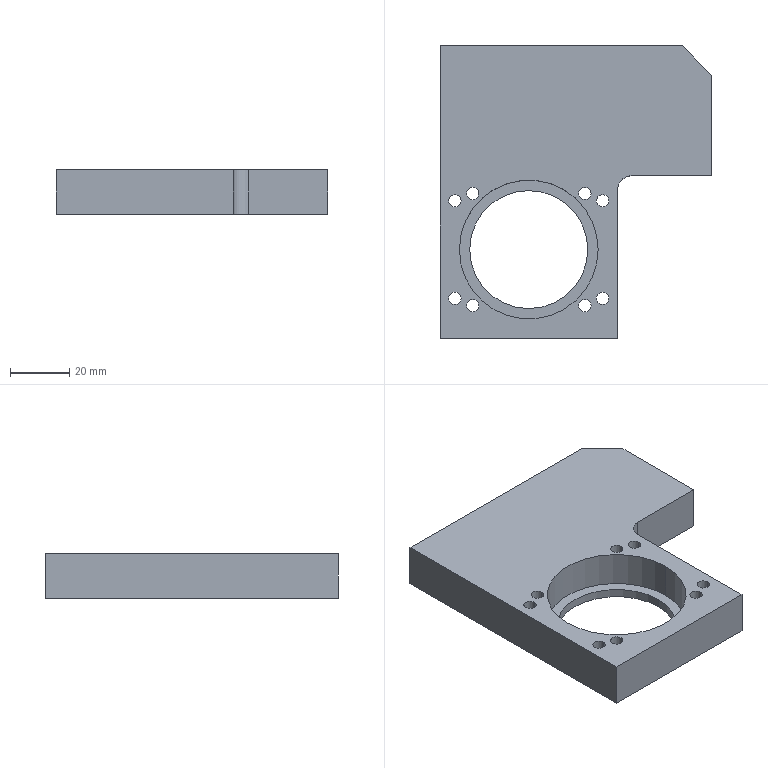Part | SolidWorks | features MirrorStock 1 | 1 solid | 55 faces | box 92 x 99 x 15 mm | volume 82233 mm3 | cylinder 33 | cone 12 | plane 10 | commonest cylinder face diameters 4.2 x28 40 x2 47 x2 10 x1